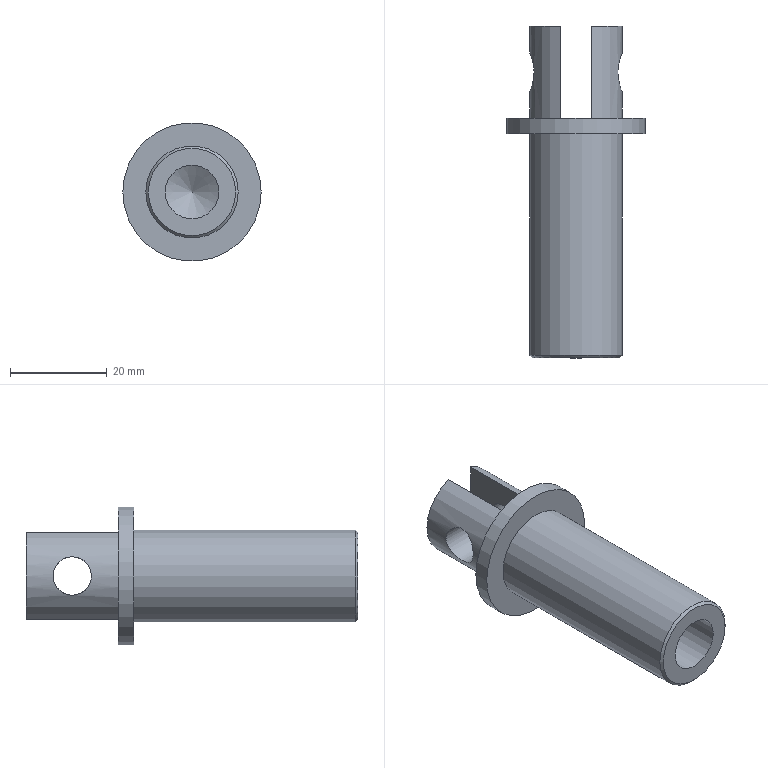Part | NX | features MG0330 trunion parts 24(stanchion group) 2 | 1 solid | 16 faces | box 28.575 x 68.517 x 28.575 mm | volume 13663 mm3 | plane 7 | cylinder 7 | cone 2 | commonest cylinder face diameters 19.05 x3 7.938 x2 11.113 x1 28.575 x1
STEP:
#1=CARTESIAN_POINT('',(3.2,33.592,8.971));
#2=VERTEX_POINT('',#1);
#3=CARTESIAN_POINT('',(3.2,33.592,-8.971));
#4=VERTEX_POINT('',#3);
#5=CARTESIAN_POINT('',(3.2,33.592,0.));
#6=DIRECTION('',(0.,0.,-1.));
#7=VECTOR('',#6,1000.);
#8=LINE('',#5,#7);
#9=EDGE_CURVE('',#2,#4,#8,.T.);
#10=ORIENTED_EDGE('',*,*,#9,.F.);
#11=CARTESIAN_POINT('',(0.,33.592,0.));
#12=DIRECTION('',(0.,-1.,0.));
#13=DIRECTION('',(1.,0.,0.));
#14=AXIS2_PLACEMENT_3D('',#11,#12,#13);
#15=CIRCLE('',#14,9.525);
#16=EDGE_CURVE('',#4,#2,#15,.T.);
#17=ORIENTED_EDGE('',*,*,#16,.F.);
#18=EDGE_LOOP('',(#10,#17));
#19=FACE_BOUND('',#18,.T.);
#20=CARTESIAN_POINT('',(9.525,33.592,0.));
#21=DIRECTION('',(0.,1.,0.));
#22=DIRECTION('',(-1.,0.,0.));
#23=AXIS2_PLACEMENT_3D('',#20,#21,#22);
#24=PLANE('',#23);
#25=ADVANCED_FACE('',(#19),#24,.T.);
#26=CARTESIAN_POINT('',(3.2,14.541,8.971));
#27=VERTEX_POINT('',#26);
#28=CARTESIAN_POINT('',(3.2,9.558,8.971));
#29=DIRECTION('',(0.,-1.,0.));
#30=VECTOR('',#29,1000.);
#31=LINE('',#28,#30);
#32=EDGE_CURVE('',#27,#2,#31,.F.);
#33=ORIENTED_EDGE('',*,*,#32,.F.);
#34=CARTESIAN_POINT('',(3.2,14.541,-8.971));
#35=VERTEX_POINT('',#34);
#36=CARTESIAN_POINT('',(0.,14.541,0.));
#37=DIRECTION('',(0.,-1.,0.));
#38=DIRECTION('',(1.,0.,0.));
#39=AXIS2_PLACEMENT_3D('',#36,#37,#38);
#40=CIRCLE('',#39,9.525);
#41=EDGE_CURVE('',#35,#27,#40,.T.);
#42=ORIENTED_EDGE('',*,*,#41,.F.);
#43=CARTESIAN_POINT('',(3.2,9.558,-8.971));
#44=DIRECTION('',(0.,-1.,0.));
#45=VECTOR('',#44,1000.);
#46=LINE('',#43,#45);
#47=EDGE_CURVE('',#4,#35,#46,.T.);
#48=ORIENTED_EDGE('',*,*,#47,.F.);
#49=ORIENTED_EDGE('',*,*,#16,.T.);
#50=EDGE_LOOP('',(#33,#42,#48,#49));
#51=FACE_BOUND('',#50,.T.);
#52=CARTESIAN_POINT('',(9.525,28.035,0.));
#53=VERTEX_POINT('',#52);
#54=CARTESIAN_POINT('',(9.111,27.174,-3.114));
#55=CARTESIAN_POINT('',(9.732,28.466,0.000635));
#56=CARTESIAN_POINT('',(9.112,27.172,3.112));
#57=CARTESIAN_POINT('',(8.432,24.075,4.398));
#58=CARTESIAN_POINT('',(9.112,20.957,3.111));
#59=CARTESIAN_POINT('',(9.731,19.668,0.007903));
#60=CARTESIAN_POINT('',(9.112,20.957,-3.112));
#61=CARTESIAN_POINT('',(8.432,24.062,-4.397));
#62=CARTESIAN_POINT('',(9.111,27.174,-3.114));
#63=CARTESIAN_POINT('',(9.732,28.466,0.000635));
#64=CARTESIAN_POINT('',(9.112,27.172,3.112));
#65=B_SPLINE_CURVE_WITH_KNOTS('',3,(#54,#55,#56,#57,#58,#59,#60,#61,#62,#63,#64),.UNSPECIFIED.,.T.,.F.,(1,1,1,1,1,1,1,1,1,1,1,1,1,1,1),(-0.009411,-0.006274,-0.003137,0.,0.003137,0.006274,0.009411,0.01255,0.01568,0.01882,0.02196,0.0251,0.02823,0.03137,0.03451),.UNSPECIFIED.);
#66=EDGE_CURVE('',#53,#53,#65,.T.);
#67=ORIENTED_EDGE('',*,*,#66,.F.);
#68=EDGE_LOOP('',(#67));
#69=FACE_BOUND('',#68,.T.);
#70=CARTESIAN_POINT('',(0.,9.558,0.));
#71=DIRECTION('',(0.,-1.,0.));
#72=DIRECTION('',(1.,0.,0.));
#73=AXIS2_PLACEMENT_3D('',#70,#71,#72);
#74=CYLINDRICAL_SURFACE('',#73,9.525);
#75=ADVANCED_FACE('',(#51,#69),#74,.T.);
#76=CARTESIAN_POINT('',(3.2,24.067,-3.969));
#77=VERTEX_POINT('',#76);
#78=CARTESIAN_POINT('',(3.2,24.067,0.));
#79=DIRECTION('',(1.,0.,0.));
#80=DIRECTION('',(0.,0.,-1.));
#81=AXIS2_PLACEMENT_3D('',#78,#79,#80);
#82=CIRCLE('',#81,3.969);
#83=EDGE_CURVE('',#77,#77,#82,.F.);
#84=ORIENTED_EDGE('',*,*,#83,.T.);
#85=EDGE_LOOP('',(#84));
#86=FACE_BOUND('',#85,.T.);
#87=ORIENTED_EDGE('',*,*,#66,.T.);
#88=EDGE_LOOP('',(#87));
#89=FACE_BOUND('',#88,.T.);
#90=CARTESIAN_POINT('',(-80.963,24.067,0.));
#91=DIRECTION('',(1.,0.,0.));
#92=DIRECTION('',(0.,0.,-1.));
#93=AXIS2_PLACEMENT_3D('',#90,#91,#92);
#94=CYLINDRICAL_SURFACE('',#93,3.969);
#95=ADVANCED_FACE('',(#86,#89),#94,.F.);
#96=CARTESIAN_POINT('',(-3.2,33.592,-8.971));
#97=VERTEX_POINT('',#96);
#98=CARTESIAN_POINT('',(-3.2,33.592,8.971));
#99=VERTEX_POINT('',#98);
#100=CARTESIAN_POINT('',(-3.2,33.592,0.));
#101=DIRECTION('',(0.,0.,1.));
#102=VECTOR('',#101,1000.);
#103=LINE('',#100,#102);
#104=EDGE_CURVE('',#97,#99,#103,.T.);
#105=ORIENTED_EDGE('',*,*,#104,.F.);
#106=CARTESIAN_POINT('',(0.,33.592,0.));
#107=DIRECTION('',(0.,-1.,0.));
#108=DIRECTION('',(1.,0.,0.));
#109=AXIS2_PLACEMENT_3D('',#106,#107,#108);
#110=CIRCLE('',#109,9.525);
#111=EDGE_CURVE('',#99,#97,#110,.T.);
#112=ORIENTED_EDGE('',*,*,#111,.F.);
#113=EDGE_LOOP('',(#105,#112));
#114=FACE_BOUND('',#113,.T.);
#115=CARTESIAN_POINT('',(9.525,33.592,0.));
#116=DIRECTION('',(0.,1.,0.));
#117=DIRECTION('',(-1.,0.,0.));
#118=AXIS2_PLACEMENT_3D('',#115,#116,#117);
#119=PLANE('',#118);
#120=ADVANCED_FACE('',(#114),#119,.T.);
#121=CARTESIAN_POINT('',(-3.2,14.541,-8.971));
#122=VERTEX_POINT('',#121);
#123=CARTESIAN_POINT('',(-3.2,9.558,-8.971));
#124=DIRECTION('',(0.,-1.,0.));
#125=VECTOR('',#124,1000.);
#126=LINE('',#123,#125);
#127=EDGE_CURVE('',#122,#97,#126,.F.);
#128=ORIENTED_EDGE('',*,*,#127,.F.);
#129=CARTESIAN_POINT('',(-3.2,14.541,8.971));
#130=VERTEX_POINT('',#129);
#131=CARTESIAN_POINT('',(0.,14.541,0.));
#132=DIRECTION('',(0.,-1.,0.));
#133=DIRECTION('',(1.,0.,0.));
#134=AXIS2_PLACEMENT_3D('',#131,#132,#133);
#135=CIRCLE('',#134,9.525);
#136=EDGE_CURVE('',#130,#122,#135,.T.);
#137=ORIENTED_EDGE('',*,*,#136,.F.);
#138=CARTESIAN_POINT('',(-3.2,9.558,8.971));
#139=DIRECTION('',(0.,-1.,0.));
#140=VECTOR('',#139,1000.);
#141=LINE('',#138,#140);
#142=EDGE_CURVE('',#99,#130,#141,.T.);
#143=ORIENTED_EDGE('',*,*,#142,.F.);
#144=ORIENTED_EDGE('',*,*,#111,.T.);
#145=EDGE_LOOP('',(#128,#137,#143,#144));
#146=FACE_BOUND('',#145,.T.);
#147=CARTESIAN_POINT('',(-8.659,24.067,-3.969));
#148=VERTEX_POINT('',#147);
#149=CARTESIAN_POINT('',(-9.113,27.177,-3.111));
#150=CARTESIAN_POINT('',(-8.432,24.066,-4.398));
#151=CARTESIAN_POINT('',(-9.112,20.958,-3.109));
#152=CARTESIAN_POINT('',(-9.731,19.667,-0.007861));
#153=CARTESIAN_POINT('',(-9.112,20.959,3.113));
#154=CARTESIAN_POINT('',(-8.432,24.059,4.397));
#155=CARTESIAN_POINT('',(-9.111,27.175,3.112));
#156=CARTESIAN_POINT('',(-9.732,28.465,0.004237));
#157=CARTESIAN_POINT('',(-9.113,27.177,-3.111));
#158=CARTESIAN_POINT('',(-8.432,24.066,-4.398));
#159=CARTESIAN_POINT('',(-9.112,20.958,-3.109));
#160=B_SPLINE_CURVE_WITH_KNOTS('',3,(#149,#150,#151,#152,#153,#154,#155,#156,#157,#158,#159),.UNSPECIFIED.,.T.,.F.,(1,1,1,1,1,1,1,1,1,1,1,1,1,1,1),(-0.00941,-0.006274,-0.003137,0.,0.003137,0.006274,0.00941,0.01255,0.01568,0.01882,0.02196,0.02509,0.02823,0.03137,0.0345),.UNSPECIFIED.);
#161=EDGE_CURVE('',#148,#148,#160,.T.);
#162=ORIENTED_EDGE('',*,*,#161,.F.);
#163=EDGE_LOOP('',(#162));
#164=FACE_BOUND('',#163,.T.);
#165=CARTESIAN_POINT('',(0.,9.558,0.));
#166=DIRECTION('',(0.,-1.,0.));
#167=DIRECTION('',(1.,0.,0.));
#168=AXIS2_PLACEMENT_3D('',#165,#166,#167);
#169=CYLINDRICAL_SURFACE('',#168,9.525);
#170=ADVANCED_FACE('',(#146,#164),#169,.T.);
#171=CARTESIAN_POINT('',(-3.2,14.541,-14.287));
#172=DIRECTION('',(0.,0.,1.));
#173=VECTOR('',#172,1000.);
#174=LINE('',#171,#173);
#175=EDGE_CURVE('',#122,#130,#174,.T.);
#176=ORIENTED_EDGE('',*,*,#175,.T.);
#177=ORIENTED_EDGE('',*,*,#136,.T.);
#178=EDGE_LOOP('',(#176,#177));
#179=FACE_BOUND('',#178,.T.);
#180=ORIENTED_EDGE('',*,*,#41,.T.);
#181=CARTESIAN_POINT('',(3.2,14.541,-14.287));
#182=DIRECTION('',(0.,0.,1.));
#183=VECTOR('',#182,1000.);
#184=LINE('',#181,#183);
#185=EDGE_CURVE('',#35,#27,#184,.T.);
#186=ORIENTED_EDGE('',*,*,#185,.F.);
#187=EDGE_LOOP('',(#180,#186));
#188=FACE_BOUND('',#187,.T.);
#189=CARTESIAN_POINT('',(14.287,14.541,0.));
#190=VERTEX_POINT('',#189);
#191=CARTESIAN_POINT('',(0.,14.541,0.));
#192=DIRECTION('',(0.,-1.,0.));
#193=DIRECTION('',(1.,0.,0.));
#194=AXIS2_PLACEMENT_3D('',#191,#192,#193);
#195=CIRCLE('',#194,14.287);
#196=EDGE_CURVE('',#190,#190,#195,.T.);
#197=ORIENTED_EDGE('',*,*,#196,.F.);
#198=EDGE_LOOP('',(#197));
#199=FACE_BOUND('',#198,.T.);
#200=CARTESIAN_POINT('',(9.525,14.541,0.));
#201=DIRECTION('',(0.,1.,0.));
#202=DIRECTION('',(-1.,0.,0.));
#203=AXIS2_PLACEMENT_3D('',#200,#201,#202);
#204=PLANE('',#203);
#205=ADVANCED_FACE('',(#179,#188,#199),#204,.T.);
#206=ORIENTED_EDGE('',*,*,#196,.T.);
#207=EDGE_LOOP('',(#206));
#208=FACE_BOUND('',#207,.T.);
#209=CARTESIAN_POINT('',(14.287,11.367,0.));
#210=VERTEX_POINT('',#209);
#211=CARTESIAN_POINT('',(0.,11.367,0.));
#212=DIRECTION('',(0.,-1.,0.));
#213=DIRECTION('',(1.,0.,0.));
#214=AXIS2_PLACEMENT_3D('',#211,#212,#213);
#215=CIRCLE('',#214,14.287);
#216=EDGE_CURVE('',#210,#210,#215,.T.);
#217=ORIENTED_EDGE('',*,*,#216,.F.);
#218=EDGE_LOOP('',(#217));
#219=FACE_BOUND('',#218,.T.);
#220=CARTESIAN_POINT('',(0.,9.558,0.));
#221=DIRECTION('',(0.,-1.,0.));
#222=DIRECTION('',(1.,0.,0.));
#223=AXIS2_PLACEMENT_3D('',#220,#221,#222);
#224=CYLINDRICAL_SURFACE('',#223,14.287);
#225=ADVANCED_FACE('',(#208,#219),#224,.T.);
#226=ORIENTED_EDGE('',*,*,#216,.T.);
#227=EDGE_LOOP('',(#226));
#228=FACE_BOUND('',#227,.T.);
#229=CARTESIAN_POINT('',(9.525,11.367,0.));
#230=VERTEX_POINT('',#229);
#231=CARTESIAN_POINT('',(0.,11.367,0.));
#232=DIRECTION('',(0.,-1.,0.));
#233=DIRECTION('',(1.,0.,0.));
#234=AXIS2_PLACEMENT_3D('',#231,#232,#233);
#235=CIRCLE('',#234,9.525);
#236=EDGE_CURVE('',#230,#230,#235,.T.);
#237=ORIENTED_EDGE('',*,*,#236,.F.);
#238=EDGE_LOOP('',(#237));
#239=FACE_BOUND('',#238,.T.);
#240=CARTESIAN_POINT('',(9.525,11.367,0.));
#241=DIRECTION('',(0.,-1.,0.));
#242=DIRECTION('',(1.,0.,0.));
#243=AXIS2_PLACEMENT_3D('',#240,#241,#242);
#244=PLANE('',#243);
#245=ADVANCED_FACE('',(#228,#239),#244,.T.);
#246=CARTESIAN_POINT('',(9.525,-34.417,0.));
#247=VERTEX_POINT('',#246);
#248=CARTESIAN_POINT('',(0.,-34.417,0.));
#249=DIRECTION('',(0.,-1.,0.));
#250=DIRECTION('',(1.,0.,0.));
#251=AXIS2_PLACEMENT_3D('',#248,#249,#250);
#252=CIRCLE('',#251,9.525);
#253=EDGE_CURVE('',#247,#247,#252,.F.);
#254=ORIENTED_EDGE('',*,*,#253,.T.);
#255=EDGE_LOOP('',(#254));
#256=FACE_BOUND('',#255,.T.);
#257=ORIENTED_EDGE('',*,*,#236,.T.);
#258=EDGE_LOOP('',(#257));
#259=FACE_BOUND('',#258,.T.);
#260=CARTESIAN_POINT('',(0.,9.558,0.));
#261=DIRECTION('',(0.,-1.,0.));
#262=DIRECTION('',(1.,0.,0.));
#263=AXIS2_PLACEMENT_3D('',#260,#261,#262);
#264=CYLINDRICAL_SURFACE('',#263,9.525);
#265=ADVANCED_FACE('',(#256,#259),#264,.T.);
#266=CARTESIAN_POINT('',(9.017,-34.925,0.));
#267=VERTEX_POINT('',#266);
#268=CARTESIAN_POINT('',(0.,-34.925,0.));
#269=DIRECTION('',(0.,-1.,0.));
#270=DIRECTION('',(1.,0.,0.));
#271=AXIS2_PLACEMENT_3D('',#268,#269,#270);
#272=CIRCLE('',#271,9.017);
#273=EDGE_CURVE('',#267,#267,#272,.T.);
#274=ORIENTED_EDGE('',*,*,#273,.T.);
#275=EDGE_LOOP('',(#274));
#276=FACE_BOUND('',#275,.T.);
#277=CARTESIAN_POINT('',(5.556,-34.925,0.));
#278=VERTEX_POINT('',#277);
#279=CARTESIAN_POINT('',(0.,-34.925,0.));
#280=DIRECTION('',(0.,-1.,0.));
#281=DIRECTION('',(1.,0.,0.));
#282=AXIS2_PLACEMENT_3D('',#279,#280,#281);
#283=CIRCLE('',#282,5.556);
#284=EDGE_CURVE('',#278,#278,#283,.T.);
#285=ORIENTED_EDGE('',*,*,#284,.F.);
#286=EDGE_LOOP('',(#285));
#287=FACE_BOUND('',#286,.T.);
#288=CARTESIAN_POINT('',(5.556,-34.925,0.));
#289=DIRECTION('',(0.,-1.,0.));
#290=DIRECTION('',(1.,0.,0.));
#291=AXIS2_PLACEMENT_3D('',#288,#289,#290);
#292=PLANE('',#291);
#293=ADVANCED_FACE('',(#276,#287),#292,.T.);
#294=ORIENTED_EDGE('',*,*,#284,.T.);
#295=EDGE_LOOP('',(#294));
#296=FACE_BOUND('',#295,.T.);
#297=CARTESIAN_POINT('',(5.556,6.35,0.));
#298=VERTEX_POINT('',#297);
#299=CARTESIAN_POINT('',(0.,6.35,0.));
#300=DIRECTION('',(0.,-1.,0.));
#301=DIRECTION('',(1.,0.,0.));
#302=AXIS2_PLACEMENT_3D('',#299,#300,#301);
#303=CIRCLE('',#302,5.556);
#304=EDGE_CURVE('',#298,#298,#303,.T.);
#305=ORIENTED_EDGE('',*,*,#304,.F.);
#306=EDGE_LOOP('',(#305));
#307=FACE_BOUND('',#306,.T.);
#308=CARTESIAN_POINT('',(0.,9.558,0.));
#309=DIRECTION('',(0.,-1.,0.));
#310=DIRECTION('',(1.,0.,0.));
#311=AXIS2_PLACEMENT_3D('',#308,#309,#310);
#312=CYLINDRICAL_SURFACE('',#311,5.556);
#313=ADVANCED_FACE('',(#296,#307),#312,.F.);
#314=ORIENTED_EDGE('',*,*,#304,.T.);
#315=EDGE_LOOP('',(#314));
#316=FACE_BOUND('',#315,.T.);
#317=CARTESIAN_POINT('',(0.,9.558,0.));
#318=VERTEX_POINT('',#317);
#319=VERTEX_LOOP('',#318);
#320=FACE_BOUND('',#319,.T.);
#321=CARTESIAN_POINT('',(0.,9.558,0.));
#322=DIRECTION('',(0.,-1.,0.));
#323=DIRECTION('',(1.,0.,0.));
#324=AXIS2_PLACEMENT_3D('',#321,#322,#323);
#325=CONICAL_SURFACE('',#324,0.,1.047);
#326=ADVANCED_FACE('',(#316,#320),#325,.F.);
#327=ORIENTED_EDGE('',*,*,#253,.F.);
#328=EDGE_LOOP('',(#327));
#329=FACE_BOUND('',#328,.T.);
#330=ORIENTED_EDGE('',*,*,#273,.F.);
#331=EDGE_LOOP('',(#330));
#332=FACE_BOUND('',#331,.T.);
#333=CARTESIAN_POINT('',(0.,-34.925,0.));
#334=DIRECTION('',(0.,1.,0.));
#335=DIRECTION('',(-1.,0.,0.));
#336=AXIS2_PLACEMENT_3D('',#333,#334,#335);
#337=CONICAL_SURFACE('',#336,9.017,0.7854);
#338=ADVANCED_FACE('',(#329,#332),#337,.T.);
#339=CARTESIAN_POINT('',(-3.2,24.067,3.969));
#340=VERTEX_POINT('',#339);
#341=CARTESIAN_POINT('',(-3.2,24.067,0.));
#342=DIRECTION('',(-1.,0.,0.));
#343=DIRECTION('',(0.,0.,1.));
#344=AXIS2_PLACEMENT_3D('',#341,#342,#343);
#345=CIRCLE('',#344,3.969);
#346=EDGE_CURVE('',#340,#340,#345,.F.);
#347=ORIENTED_EDGE('',*,*,#346,.T.);
#348=EDGE_LOOP('',(#347));
#349=FACE_BOUND('',#348,.T.);
#350=ORIENTED_EDGE('',*,*,#161,.T.);
#351=EDGE_LOOP('',(#350));
#352=FACE_BOUND('',#351,.T.);
#353=CARTESIAN_POINT('',(-80.963,24.067,0.));
#354=DIRECTION('',(1.,0.,0.));
#355=DIRECTION('',(0.,0.,-1.));
#356=AXIS2_PLACEMENT_3D('',#353,#354,#355);
#357=CYLINDRICAL_SURFACE('',#356,3.969);
#358=ADVANCED_FACE('',(#349,#352),#357,.F.);
#359=ORIENTED_EDGE('',*,*,#32,.T.);
#360=ORIENTED_EDGE('',*,*,#9,.T.);
#361=ORIENTED_EDGE('',*,*,#47,.T.);
#362=ORIENTED_EDGE('',*,*,#185,.T.);
#363=EDGE_LOOP('',(#359,#360,#361,#362));
#364=FACE_BOUND('',#363,.T.);
#365=ORIENTED_EDGE('',*,*,#83,.F.);
#366=EDGE_LOOP('',(#365));
#367=FACE_BOUND('',#366,.T.);
#368=CARTESIAN_POINT('',(3.2,14.541,-14.287));
#369=DIRECTION('',(1.,0.,0.));
#370=DIRECTION('',(0.,0.,-1.));
#371=AXIS2_PLACEMENT_3D('',#368,#369,#370);
#372=PLANE('',#371);
#373=ADVANCED_FACE('',(#364,#367),#372,.F.);
#374=ORIENTED_EDGE('',*,*,#127,.T.);
#375=ORIENTED_EDGE('',*,*,#104,.T.);
#376=ORIENTED_EDGE('',*,*,#142,.T.);
#377=ORIENTED_EDGE('',*,*,#175,.F.);
#378=EDGE_LOOP('',(#374,#375,#376,#377));
#379=FACE_BOUND('',#378,.T.);
#380=ORIENTED_EDGE('',*,*,#346,.F.);
#381=EDGE_LOOP('',(#380));
#382=FACE_BOUND('',#381,.T.);
#383=CARTESIAN_POINT('',(-3.2,14.541,-14.287));
#384=DIRECTION('',(-1.,0.,0.));
#385=DIRECTION('',(0.,0.,1.));
#386=AXIS2_PLACEMENT_3D('',#383,#384,#385);
#387=PLANE('',#386);
#388=ADVANCED_FACE('',(#379,#382),#387,.F.);
#389=CLOSED_SHELL('',(#25,#75,#95,#120,#170,#205,#225,#245,#265,#293,#313,#326,#338,#358,#373,#388));
#390=MANIFOLD_SOLID_BREP('',#389);
#391=(LENGTH_UNIT()NAMED_UNIT(*)SI_UNIT(.MILLI.,.METRE.));
#392=UNCERTAINTY_MEASURE_WITH_UNIT(LENGTH_MEASURE(0.0508),#391,'','');
#393=(NAMED_UNIT(*)PLANE_ANGLE_UNIT()SI_UNIT($,.RADIAN.));
#394=(NAMED_UNIT(*)SI_UNIT($,.STERADIAN.)SOLID_ANGLE_UNIT());
#395=(GEOMETRIC_REPRESENTATION_CONTEXT(3)GLOBAL_UNCERTAINTY_ASSIGNED_CONTEXT((#392))GLOBAL_UNIT_ASSIGNED_CONTEXT((#391,#393,#394))REPRESENTATION_CONTEXT('',''));
#396=ADVANCED_BREP_SHAPE_REPRESENTATION('',(#390),#395);